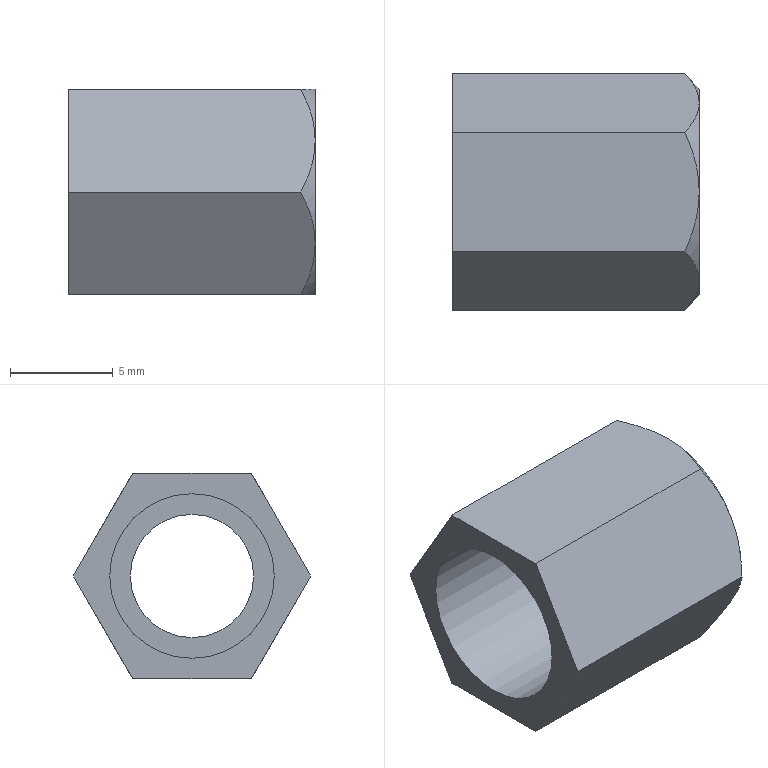Part | STEP file | 1-75.3 | 2 solids | 21 faces | box 12 x 11.547 x 10 mm | volume 521.946 mm3 | plane 11 | cone 6 | cylinder 4 | commonest cylinder face diameters 6 x2 8 x2